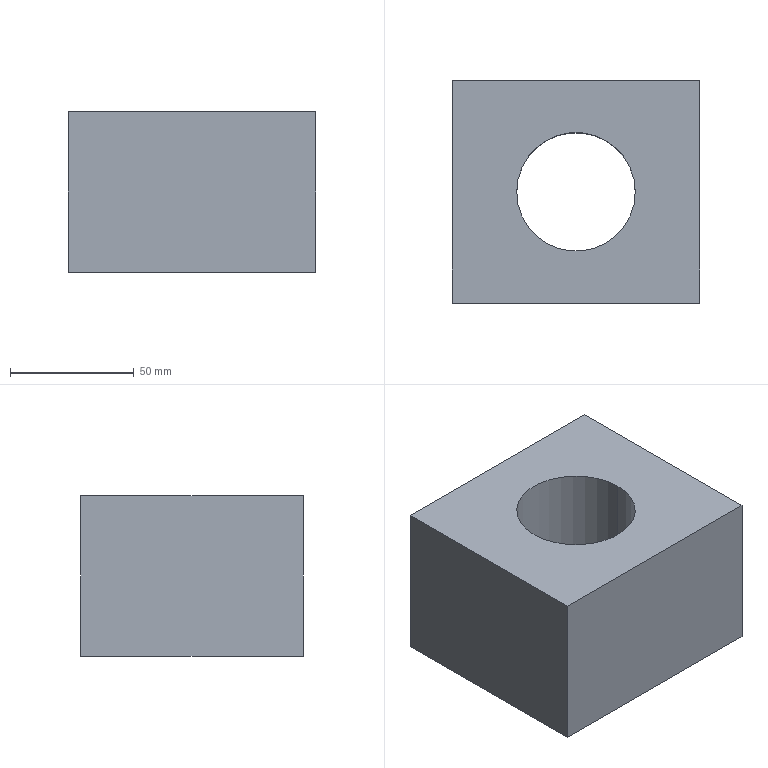Part | SolidWorks | features Extrusion 1 | 1 solid | 8 faces | box 100 x 90 x 65 mm | volume 467379 mm3 | plane 6 | cylinder 2 | commonest cylinder face diameters 48 x2
STEP:
#1=CARTESIAN_POINT('',(26.,45.,65.));
#2=VERTEX_POINT('',#1);
#3=CARTESIAN_POINT('',(74.,45.,65.));
#4=VERTEX_POINT('',#3);
#5=CARTESIAN_POINT('',(50.,45.,65.));
#6=DIRECTION('',(0.,0.,1.));
#7=DIRECTION('',(1.,0.,0.));
#8=AXIS2_PLACEMENT_3D('',#5,#6,#7);
#9=CIRCLE('',#8,24.);
#10=EDGE_CURVE('',#2,#4,#9,.T.);
#11=ORIENTED_EDGE('',*,*,#10,.T.);
#12=CARTESIAN_POINT('',(74.,45.,0.));
#13=VERTEX_POINT('',#12);
#14=CARTESIAN_POINT('',(74.,45.,65.));
#15=DIRECTION('',(0.,0.,-1.));
#16=VECTOR('',#15,1000.);
#17=LINE('',#14,#16);
#18=EDGE_CURVE('',#4,#13,#17,.T.);
#19=ORIENTED_EDGE('',*,*,#18,.T.);
#20=CARTESIAN_POINT('',(26.,45.,0.));
#21=VERTEX_POINT('',#20);
#22=CARTESIAN_POINT('',(50.,45.,0.));
#23=DIRECTION('',(0.,0.,1.));
#24=DIRECTION('',(1.,0.,0.));
#25=AXIS2_PLACEMENT_3D('',#22,#23,#24);
#26=CIRCLE('',#25,24.);
#27=EDGE_CURVE('',#21,#13,#26,.T.);
#28=ORIENTED_EDGE('',*,*,#27,.F.);
#29=CARTESIAN_POINT('',(26.,45.,65.));
#30=DIRECTION('',(0.,0.,-1.));
#31=VECTOR('',#30,1000.);
#32=LINE('',#29,#31);
#33=EDGE_CURVE('',#2,#21,#32,.T.);
#34=ORIENTED_EDGE('',*,*,#33,.F.);
#35=EDGE_LOOP('',(#11,#19,#28,#34));
#36=FACE_OUTER_BOUND('',#35,.T.);
#37=CARTESIAN_POINT('',(50.,45.,65.));
#38=DIRECTION('',(0.,0.,-1.));
#39=DIRECTION('',(-1.,0.,0.));
#40=AXIS2_PLACEMENT_3D('',#37,#38,#39);
#41=CYLINDRICAL_SURFACE('',#40,24.);
#42=ADVANCED_FACE('',(#36),#41,.F.);
#43=CARTESIAN_POINT('',(0.,90.,65.));
#44=VERTEX_POINT('',#43);
#45=CARTESIAN_POINT('',(0.,0.,65.));
#46=VERTEX_POINT('',#45);
#47=CARTESIAN_POINT('',(0.,0.,65.));
#48=DIRECTION('',(0.,-1.,0.));
#49=VECTOR('',#48,1000.);
#50=LINE('',#47,#49);
#51=EDGE_CURVE('',#44,#46,#50,.T.);
#52=ORIENTED_EDGE('',*,*,#51,.T.);
#53=CARTESIAN_POINT('',(100.,0.,65.));
#54=VERTEX_POINT('',#53);
#55=CARTESIAN_POINT('',(0.,0.,65.));
#56=DIRECTION('',(1.,0.,0.));
#57=VECTOR('',#56,1000.);
#58=LINE('',#55,#57);
#59=EDGE_CURVE('',#46,#54,#58,.T.);
#60=ORIENTED_EDGE('',*,*,#59,.T.);
#61=CARTESIAN_POINT('',(100.,90.,65.));
#62=VERTEX_POINT('',#61);
#63=CARTESIAN_POINT('',(100.,0.,65.));
#64=DIRECTION('',(0.,1.,0.));
#65=VECTOR('',#64,1000.);
#66=LINE('',#63,#65);
#67=EDGE_CURVE('',#54,#62,#66,.T.);
#68=ORIENTED_EDGE('',*,*,#67,.T.);
#69=CARTESIAN_POINT('',(0.,90.,65.));
#70=DIRECTION('',(-1.,0.,0.));
#71=VECTOR('',#70,1000.);
#72=LINE('',#69,#71);
#73=EDGE_CURVE('',#62,#44,#72,.T.);
#74=ORIENTED_EDGE('',*,*,#73,.T.);
#75=EDGE_LOOP('',(#52,#60,#68,#74));
#76=FACE_OUTER_BOUND('',#75,.T.);
#77=ORIENTED_EDGE('',*,*,#10,.F.);
#78=CARTESIAN_POINT('',(50.,45.,65.));
#79=DIRECTION('',(0.,0.,1.));
#80=DIRECTION('',(1.,0.,0.));
#81=AXIS2_PLACEMENT_3D('',#78,#79,#80);
#82=CIRCLE('',#81,24.);
#83=EDGE_CURVE('',#4,#2,#82,.T.);
#84=ORIENTED_EDGE('',*,*,#83,.F.);
#85=EDGE_LOOP('',(#77,#84));
#86=FACE_BOUND('',#85,.T.);
#87=CARTESIAN_POINT('',(0.,0.,65.));
#88=DIRECTION('',(0.,0.,-1.));
#89=DIRECTION('',(-1.,0.,0.));
#90=AXIS2_PLACEMENT_3D('',#87,#88,#89);
#91=PLANE('',#90);
#92=ADVANCED_FACE('',(#76,#86),#91,.F.);
#93=CARTESIAN_POINT('',(0.,90.,0.));
#94=VERTEX_POINT('',#93);
#95=CARTESIAN_POINT('',(0.,0.,0.));
#96=VERTEX_POINT('',#95);
#97=CARTESIAN_POINT('',(0.,0.,0.));
#98=DIRECTION('',(0.,-1.,0.));
#99=VECTOR('',#98,1000.);
#100=LINE('',#97,#99);
#101=EDGE_CURVE('',#94,#96,#100,.T.);
#102=ORIENTED_EDGE('',*,*,#101,.F.);
#103=CARTESIAN_POINT('',(100.,90.,0.));
#104=VERTEX_POINT('',#103);
#105=CARTESIAN_POINT('',(0.,90.,0.));
#106=DIRECTION('',(-1.,0.,0.));
#107=VECTOR('',#106,1000.);
#108=LINE('',#105,#107);
#109=EDGE_CURVE('',#104,#94,#108,.T.);
#110=ORIENTED_EDGE('',*,*,#109,.F.);
#111=CARTESIAN_POINT('',(100.,0.,0.));
#112=VERTEX_POINT('',#111);
#113=CARTESIAN_POINT('',(100.,0.,0.));
#114=DIRECTION('',(0.,1.,0.));
#115=VECTOR('',#114,1000.);
#116=LINE('',#113,#115);
#117=EDGE_CURVE('',#112,#104,#116,.T.);
#118=ORIENTED_EDGE('',*,*,#117,.F.);
#119=CARTESIAN_POINT('',(0.,0.,0.));
#120=DIRECTION('',(1.,0.,0.));
#121=VECTOR('',#120,1000.);
#122=LINE('',#119,#121);
#123=EDGE_CURVE('',#96,#112,#122,.T.);
#124=ORIENTED_EDGE('',*,*,#123,.F.);
#125=EDGE_LOOP('',(#102,#110,#118,#124));
#126=FACE_OUTER_BOUND('',#125,.T.);
#127=ORIENTED_EDGE('',*,*,#27,.T.);
#128=CARTESIAN_POINT('',(50.,45.,0.));
#129=DIRECTION('',(0.,0.,1.));
#130=DIRECTION('',(1.,0.,0.));
#131=AXIS2_PLACEMENT_3D('',#128,#129,#130);
#132=CIRCLE('',#131,24.);
#133=EDGE_CURVE('',#13,#21,#132,.T.);
#134=ORIENTED_EDGE('',*,*,#133,.T.);
#135=EDGE_LOOP('',(#127,#134));
#136=FACE_BOUND('',#135,.T.);
#137=CARTESIAN_POINT('',(0.,0.,0.));
#138=DIRECTION('',(0.,0.,-1.));
#139=DIRECTION('',(-1.,0.,0.));
#140=AXIS2_PLACEMENT_3D('',#137,#138,#139);
#141=PLANE('',#140);
#142=ADVANCED_FACE('',(#126,#136),#141,.T.);
#143=ORIENTED_EDGE('',*,*,#101,.T.);
#144=CARTESIAN_POINT('',(0.,0.,65.));
#145=DIRECTION('',(0.,0.,-1.));
#146=VECTOR('',#145,1000.);
#147=LINE('',#144,#146);
#148=EDGE_CURVE('',#46,#96,#147,.T.);
#149=ORIENTED_EDGE('',*,*,#148,.F.);
#150=ORIENTED_EDGE('',*,*,#51,.F.);
#151=CARTESIAN_POINT('',(0.,90.,65.));
#152=DIRECTION('',(0.,0.,-1.));
#153=VECTOR('',#152,1000.);
#154=LINE('',#151,#153);
#155=EDGE_CURVE('',#44,#94,#154,.T.);
#156=ORIENTED_EDGE('',*,*,#155,.T.);
#157=EDGE_LOOP('',(#143,#149,#150,#156));
#158=FACE_OUTER_BOUND('',#157,.T.);
#159=CARTESIAN_POINT('',(0.,0.,65.));
#160=DIRECTION('',(1.,0.,0.));
#161=DIRECTION('',(0.,0.,-1.));
#162=AXIS2_PLACEMENT_3D('',#159,#160,#161);
#163=PLANE('',#162);
#164=ADVANCED_FACE('',(#158),#163,.F.);
#165=ORIENTED_EDGE('',*,*,#123,.T.);
#166=CARTESIAN_POINT('',(100.,0.,65.));
#167=DIRECTION('',(0.,0.,-1.));
#168=VECTOR('',#167,1000.);
#169=LINE('',#166,#168);
#170=EDGE_CURVE('',#54,#112,#169,.T.);
#171=ORIENTED_EDGE('',*,*,#170,.F.);
#172=ORIENTED_EDGE('',*,*,#59,.F.);
#173=ORIENTED_EDGE('',*,*,#148,.T.);
#174=EDGE_LOOP('',(#165,#171,#172,#173));
#175=FACE_OUTER_BOUND('',#174,.T.);
#176=CARTESIAN_POINT('',(0.,0.,65.));
#177=DIRECTION('',(0.,1.,0.));
#178=DIRECTION('',(0.,0.,1.));
#179=AXIS2_PLACEMENT_3D('',#176,#177,#178);
#180=PLANE('',#179);
#181=ADVANCED_FACE('',(#175),#180,.F.);
#182=ORIENTED_EDGE('',*,*,#117,.T.);
#183=CARTESIAN_POINT('',(100.,90.,65.));
#184=DIRECTION('',(0.,0.,-1.));
#185=VECTOR('',#184,1000.);
#186=LINE('',#183,#185);
#187=EDGE_CURVE('',#62,#104,#186,.T.);
#188=ORIENTED_EDGE('',*,*,#187,.F.);
#189=ORIENTED_EDGE('',*,*,#67,.F.);
#190=ORIENTED_EDGE('',*,*,#170,.T.);
#191=EDGE_LOOP('',(#182,#188,#189,#190));
#192=FACE_OUTER_BOUND('',#191,.T.);
#193=CARTESIAN_POINT('',(100.,0.,65.));
#194=DIRECTION('',(-1.,0.,0.));
#195=DIRECTION('',(0.,0.,1.));
#196=AXIS2_PLACEMENT_3D('',#193,#194,#195);
#197=PLANE('',#196);
#198=ADVANCED_FACE('',(#192),#197,.F.);
#199=ORIENTED_EDGE('',*,*,#109,.T.);
#200=ORIENTED_EDGE('',*,*,#155,.F.);
#201=ORIENTED_EDGE('',*,*,#73,.F.);
#202=ORIENTED_EDGE('',*,*,#187,.T.);
#203=EDGE_LOOP('',(#199,#200,#201,#202));
#204=FACE_OUTER_BOUND('',#203,.T.);
#205=CARTESIAN_POINT('',(0.,90.,65.));
#206=DIRECTION('',(0.,-1.,0.));
#207=DIRECTION('',(0.,0.,-1.));
#208=AXIS2_PLACEMENT_3D('',#205,#206,#207);
#209=PLANE('',#208);
#210=ADVANCED_FACE('',(#204),#209,.F.);
#211=ORIENTED_EDGE('',*,*,#18,.F.);
#212=ORIENTED_EDGE('',*,*,#83,.T.);
#213=ORIENTED_EDGE('',*,*,#33,.T.);
#214=ORIENTED_EDGE('',*,*,#133,.F.);
#215=EDGE_LOOP('',(#211,#212,#213,#214));
#216=FACE_OUTER_BOUND('',#215,.T.);
#217=CARTESIAN_POINT('',(50.,45.,65.));
#218=DIRECTION('',(0.,0.,-1.));
#219=DIRECTION('',(-1.,0.,0.));
#220=AXIS2_PLACEMENT_3D('',#217,#218,#219);
#221=CYLINDRICAL_SURFACE('',#220,24.);
#222=ADVANCED_FACE('',(#216),#221,.F.);
#223=CLOSED_SHELL('',(#42,#92,#142,#164,#181,#198,#210,#222));
#224=MANIFOLD_SOLID_BREP('',#223);
#225=CARTESIAN_POINT('',(0.,0.,0.));
#226=DIRECTION('',(0.,0.,1.));
#227=DIRECTION('',(1.,0.,0.));
#228=AXIS2_PLACEMENT_3D('',#225,#226,#227);
#229=(LENGTH_UNIT()NAMED_UNIT(*)SI_UNIT(.MILLI.,.METRE.));
#230=UNCERTAINTY_MEASURE_WITH_UNIT(LENGTH_MEASURE(0.00001),#229,'','');
#231=(NAMED_UNIT(*)PLANE_ANGLE_UNIT()SI_UNIT($,.RADIAN.));
#232=(NAMED_UNIT(*)SI_UNIT($,.STERADIAN.)SOLID_ANGLE_UNIT());
#233=(GEOMETRIC_REPRESENTATION_CONTEXT(3)GLOBAL_UNCERTAINTY_ASSIGNED_CONTEXT((#230))GLOBAL_UNIT_ASSIGNED_CONTEXT((#229,#231,#232))REPRESENTATION_CONTEXT('',''));
#234=ADVANCED_BREP_SHAPE_REPRESENTATION('',(#224,#228),#233);